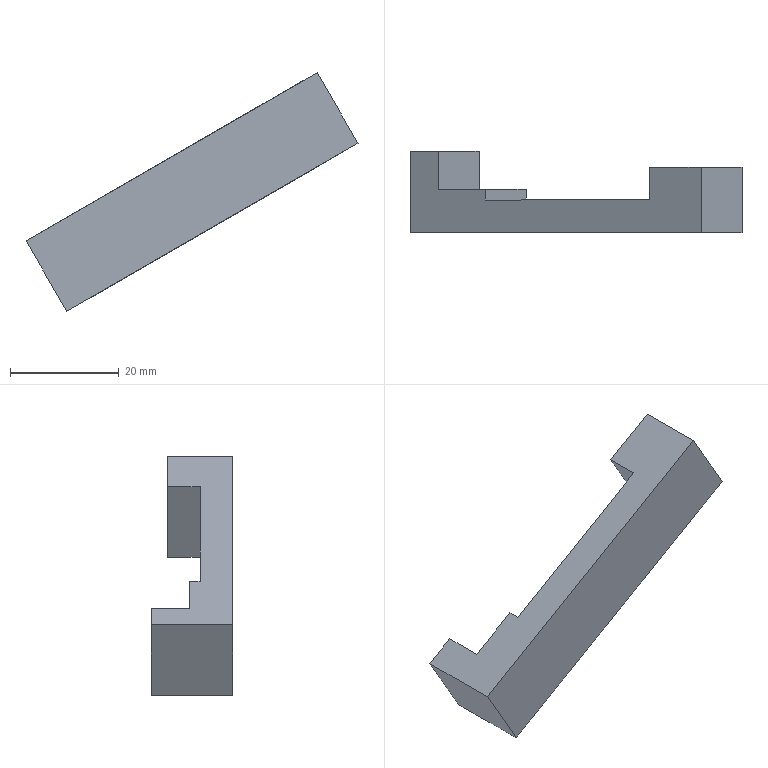Part | NX | features solid 2 | 1 solid | 12 faces | box 61.034 x 15 x 43.898 mm | volume 7663 mm3 | plane 12
STEP:
#1=CARTESIAN_POINT('',(16.962,672.,239.949));
#2=VERTEX_POINT('',#1);
#3=CARTESIAN_POINT('',(9.462,672.,252.94));
#4=VERTEX_POINT('',#3);
#5=CARTESIAN_POINT('',(16.962,672.,239.949));
#6=DIRECTION('',(0.5,0.,-0.866));
#7=VECTOR('',#6,1000.);
#8=LINE('',#5,#7);
#9=EDGE_CURVE('',#2,#4,#8,.F.);
#10=ORIENTED_EDGE('',*,*,#9,.F.);
#11=CARTESIAN_POINT('',(-13.189,672.,222.542));
#12=VERTEX_POINT('',#11);
#13=CARTESIAN_POINT('',(26.488,672.,245.449));
#14=DIRECTION('',(-0.866,0.,-0.5));
#15=VECTOR('',#14,1000.);
#16=LINE('',#13,#15);
#17=EDGE_CURVE('',#2,#12,#16,.T.);
#18=ORIENTED_EDGE('',*,*,#17,.T.);
#19=CARTESIAN_POINT('',(-20.689,672.,235.532));
#20=VERTEX_POINT('',#19);
#21=CARTESIAN_POINT('',(-13.189,672.,222.542));
#22=DIRECTION('',(-0.5,0.,0.866));
#23=VECTOR('',#22,1000.);
#24=LINE('',#21,#23);
#25=EDGE_CURVE('',#12,#20,#24,.T.);
#26=ORIENTED_EDGE('',*,*,#25,.T.);
#27=CARTESIAN_POINT('',(18.988,672.,258.44));
#28=DIRECTION('',(-0.866,0.,-0.5));
#29=VECTOR('',#28,1000.);
#30=LINE('',#27,#29);
#31=EDGE_CURVE('',#4,#20,#30,.T.);
#32=ORIENTED_EDGE('',*,*,#31,.F.);
#33=EDGE_LOOP('',(#10,#18,#26,#32));
#34=FACE_BOUND('',#33,.T.);
#35=CARTESIAN_POINT('',(11.488,672.,271.43));
#36=DIRECTION('',(0.,-1.,0.));
#37=DIRECTION('',(-0.866,0.,-0.5));
#38=AXIS2_PLACEMENT_3D('',#35,#36,#37);
#39=PLANE('',#38);
#40=ADVANCED_FACE('',(#34),#39,.F.);
#41=CARTESIAN_POINT('',(26.488,666.,245.449));
#42=VERTEX_POINT('',#41);
#43=CARTESIAN_POINT('',(18.988,666.,258.44));
#44=VERTEX_POINT('',#43);
#45=CARTESIAN_POINT('',(11.488,666.,271.43));
#46=DIRECTION('',(0.5,0.,-0.866));
#47=VECTOR('',#46,1000.);
#48=LINE('',#45,#47);
#49=EDGE_CURVE('',#42,#44,#48,.F.);
#50=ORIENTED_EDGE('',*,*,#49,.T.);
#51=CARTESIAN_POINT('',(-34.545,666.,227.532));
#52=VERTEX_POINT('',#51);
#53=CARTESIAN_POINT('',(18.988,666.,258.44));
#54=DIRECTION('',(-0.866,0.,-0.5));
#55=VECTOR('',#54,1000.);
#56=LINE('',#53,#55);
#57=EDGE_CURVE('',#44,#52,#56,.T.);
#58=ORIENTED_EDGE('',*,*,#57,.T.);
#59=CARTESIAN_POINT('',(-27.045,666.,214.542));
#60=VERTEX_POINT('',#59);
#61=CARTESIAN_POINT('',(-42.045,666.,240.522));
#62=DIRECTION('',(-0.5,0.,0.866));
#63=VECTOR('',#62,1000.);
#64=LINE('',#61,#63);
#65=EDGE_CURVE('',#60,#52,#64,.T.);
#66=ORIENTED_EDGE('',*,*,#65,.F.);
#67=CARTESIAN_POINT('',(26.488,666.,245.449));
#68=DIRECTION('',(-0.866,0.,-0.5));
#69=VECTOR('',#68,1000.);
#70=LINE('',#67,#69);
#71=EDGE_CURVE('',#42,#60,#70,.T.);
#72=ORIENTED_EDGE('',*,*,#71,.F.);
#73=EDGE_LOOP('',(#50,#58,#66,#72));
#74=FACE_BOUND('',#73,.T.);
#75=CARTESIAN_POINT('',(11.488,666.,271.43));
#76=DIRECTION('',(0.,-1.,0.));
#77=DIRECTION('',(-0.866,0.,-0.5));
#78=AXIS2_PLACEMENT_3D('',#75,#76,#77);
#79=PLANE('',#78);
#80=ADVANCED_FACE('',(#74),#79,.T.);
#81=ORIENTED_EDGE('',*,*,#65,.T.);
#82=CARTESIAN_POINT('',(-34.545,681.,227.532));
#83=VERTEX_POINT('',#82);
#84=CARTESIAN_POINT('',(-34.545,666.,227.532));
#85=DIRECTION('',(0.,-1.,0.));
#86=VECTOR('',#85,1000.);
#87=LINE('',#84,#86);
#88=EDGE_CURVE('',#52,#83,#87,.F.);
#89=ORIENTED_EDGE('',*,*,#88,.T.);
#90=CARTESIAN_POINT('',(-27.045,681.,214.542));
#91=VERTEX_POINT('',#90);
#92=CARTESIAN_POINT('',(-27.045,681.,214.542));
#93=DIRECTION('',(-0.5,0.,0.866));
#94=VECTOR('',#93,1000.);
#95=LINE('',#92,#94);
#96=EDGE_CURVE('',#91,#83,#95,.T.);
#97=ORIENTED_EDGE('',*,*,#96,.F.);
#98=CARTESIAN_POINT('',(-27.045,666.,214.542));
#99=DIRECTION('',(0.,-1.,0.));
#100=VECTOR('',#99,1000.);
#101=LINE('',#98,#100);
#102=EDGE_CURVE('',#60,#91,#101,.F.);
#103=ORIENTED_EDGE('',*,*,#102,.F.);
#104=EDGE_LOOP('',(#81,#89,#97,#103));
#105=FACE_BOUND('',#104,.T.);
#106=CARTESIAN_POINT('',(-42.045,666.,240.522));
#107=DIRECTION('',(-0.866,0.,-0.5));
#108=DIRECTION('',(0.,1.,0.));
#109=AXIS2_PLACEMENT_3D('',#106,#107,#108);
#110=PLANE('',#109);
#111=ADVANCED_FACE('',(#105),#110,.T.);
#112=CARTESIAN_POINT('',(26.488,678.,245.449));
#113=VERTEX_POINT('',#112);
#114=CARTESIAN_POINT('',(26.488,666.,245.449));
#115=DIRECTION('',(0.,1.,0.));
#116=VECTOR('',#115,1000.);
#117=LINE('',#114,#116);
#118=EDGE_CURVE('',#42,#113,#117,.T.);
#119=ORIENTED_EDGE('',*,*,#118,.T.);
#120=CARTESIAN_POINT('',(18.988,678.,258.44));
#121=VERTEX_POINT('',#120);
#122=CARTESIAN_POINT('',(26.488,678.,245.449));
#123=DIRECTION('',(-0.5,0.,0.866));
#124=VECTOR('',#123,1000.);
#125=LINE('',#122,#124);
#126=EDGE_CURVE('',#113,#121,#125,.T.);
#127=ORIENTED_EDGE('',*,*,#126,.T.);
#128=CARTESIAN_POINT('',(18.988,666.,258.44));
#129=DIRECTION('',(0.,1.,0.));
#130=VECTOR('',#129,1000.);
#131=LINE('',#128,#130);
#132=EDGE_CURVE('',#44,#121,#131,.T.);
#133=ORIENTED_EDGE('',*,*,#132,.F.);
#134=ORIENTED_EDGE('',*,*,#49,.F.);
#135=EDGE_LOOP('',(#119,#127,#133,#134));
#136=FACE_BOUND('',#135,.T.);
#137=CARTESIAN_POINT('',(11.488,666.,271.43));
#138=DIRECTION('',(-0.866,0.,-0.5));
#139=DIRECTION('',(0.,1.,0.));
#140=AXIS2_PLACEMENT_3D('',#137,#138,#139);
#141=PLANE('',#140);
#142=ADVANCED_FACE('',(#136),#141,.F.);
#143=CARTESIAN_POINT('',(-29.349,681.,230.532));
#144=VERTEX_POINT('',#143);
#145=CARTESIAN_POINT('',(-29.349,681.,230.532));
#146=DIRECTION('',(-0.866,0.,-0.5));
#147=VECTOR('',#146,1000.);
#148=LINE('',#145,#147);
#149=EDGE_CURVE('',#144,#83,#148,.T.);
#150=ORIENTED_EDGE('',*,*,#149,.T.);
#151=ORIENTED_EDGE('',*,*,#88,.F.);
#152=ORIENTED_EDGE('',*,*,#57,.F.);
#153=ORIENTED_EDGE('',*,*,#132,.T.);
#154=CARTESIAN_POINT('',(9.462,678.,252.94));
#155=VERTEX_POINT('',#154);
#156=CARTESIAN_POINT('',(18.988,678.,258.44));
#157=DIRECTION('',(0.866,0.,0.5));
#158=VECTOR('',#157,1000.);
#159=LINE('',#156,#158);
#160=EDGE_CURVE('',#121,#155,#159,.F.);
#161=ORIENTED_EDGE('',*,*,#160,.T.);
#162=CARTESIAN_POINT('',(9.462,678.,252.94));
#163=DIRECTION('',(0.,1.,0.));
#164=VECTOR('',#163,1000.);
#165=LINE('',#162,#164);
#166=EDGE_CURVE('',#155,#4,#165,.F.);
#167=ORIENTED_EDGE('',*,*,#166,.T.);
#168=ORIENTED_EDGE('',*,*,#31,.T.);
#169=CARTESIAN_POINT('',(-20.689,674.,235.532));
#170=VERTEX_POINT('',#169);
#171=CARTESIAN_POINT('',(-20.689,672.,235.532));
#172=DIRECTION('',(0.,1.,0.));
#173=VECTOR('',#172,1000.);
#174=LINE('',#171,#173);
#175=EDGE_CURVE('',#20,#170,#174,.T.);
#176=ORIENTED_EDGE('',*,*,#175,.T.);
#177=CARTESIAN_POINT('',(-29.349,674.,230.532));
#178=VERTEX_POINT('',#177);
#179=CARTESIAN_POINT('',(-20.689,674.,235.532));
#180=DIRECTION('',(-0.866,0.,-0.5));
#181=VECTOR('',#180,1000.);
#182=LINE('',#179,#181);
#183=EDGE_CURVE('',#170,#178,#182,.T.);
#184=ORIENTED_EDGE('',*,*,#183,.T.);
#185=CARTESIAN_POINT('',(-29.349,672.,230.532));
#186=DIRECTION('',(0.,1.,0.));
#187=VECTOR('',#186,1000.);
#188=LINE('',#185,#187);
#189=EDGE_CURVE('',#178,#144,#188,.T.);
#190=ORIENTED_EDGE('',*,*,#189,.T.);
#191=EDGE_LOOP('',(#150,#151,#152,#153,#161,#167,#168,#176,#184,#190));
#192=FACE_BOUND('',#191,.T.);
#193=CARTESIAN_POINT('',(18.988,666.,258.44));
#194=DIRECTION('',(0.5,0.,-0.866));
#195=DIRECTION('',(-0.866,0.,-0.5));
#196=AXIS2_PLACEMENT_3D('',#193,#194,#195);
#197=PLANE('',#196);
#198=ADVANCED_FACE('',(#192),#197,.F.);
#199=ORIENTED_EDGE('',*,*,#102,.T.);
#200=CARTESIAN_POINT('',(-21.849,681.,217.542));
#201=VERTEX_POINT('',#200);
#202=CARTESIAN_POINT('',(-21.849,681.,217.542));
#203=DIRECTION('',(-0.866,0.,-0.5));
#204=VECTOR('',#203,1000.);
#205=LINE('',#202,#204);
#206=EDGE_CURVE('',#201,#91,#205,.T.);
#207=ORIENTED_EDGE('',*,*,#206,.F.);
#208=CARTESIAN_POINT('',(-21.849,674.,217.542));
#209=VERTEX_POINT('',#208);
#210=CARTESIAN_POINT('',(-21.849,672.,217.542));
#211=DIRECTION('',(0.,1.,0.));
#212=VECTOR('',#211,1000.);
#213=LINE('',#210,#212);
#214=EDGE_CURVE('',#209,#201,#213,.T.);
#215=ORIENTED_EDGE('',*,*,#214,.F.);
#216=CARTESIAN_POINT('',(-13.189,674.,222.542));
#217=VERTEX_POINT('',#216);
#218=CARTESIAN_POINT('',(-13.189,674.,222.542));
#219=DIRECTION('',(-0.866,0.,-0.5));
#220=VECTOR('',#219,1000.);
#221=LINE('',#218,#220);
#222=EDGE_CURVE('',#217,#209,#221,.T.);
#223=ORIENTED_EDGE('',*,*,#222,.F.);
#224=CARTESIAN_POINT('',(-13.189,672.,222.542));
#225=DIRECTION('',(0.,1.,0.));
#226=VECTOR('',#225,1000.);
#227=LINE('',#224,#226);
#228=EDGE_CURVE('',#12,#217,#227,.T.);
#229=ORIENTED_EDGE('',*,*,#228,.F.);
#230=ORIENTED_EDGE('',*,*,#17,.F.);
#231=CARTESIAN_POINT('',(16.962,678.,239.949));
#232=VERTEX_POINT('',#231);
#233=CARTESIAN_POINT('',(16.962,678.,239.949));
#234=DIRECTION('',(0.,1.,0.));
#235=VECTOR('',#234,1000.);
#236=LINE('',#233,#235);
#237=EDGE_CURVE('',#232,#2,#236,.F.);
#238=ORIENTED_EDGE('',*,*,#237,.F.);
#239=CARTESIAN_POINT('',(26.488,678.,245.449));
#240=DIRECTION('',(0.866,0.,0.5));
#241=VECTOR('',#240,1000.);
#242=LINE('',#239,#241);
#243=EDGE_CURVE('',#113,#232,#242,.F.);
#244=ORIENTED_EDGE('',*,*,#243,.F.);
#245=ORIENTED_EDGE('',*,*,#118,.F.);
#246=ORIENTED_EDGE('',*,*,#71,.T.);
#247=EDGE_LOOP('',(#199,#207,#215,#223,#229,#230,#238,#244,#245,#246));
#248=FACE_BOUND('',#247,.T.);
#249=CARTESIAN_POINT('',(26.488,666.,245.449));
#250=DIRECTION('',(0.5,0.,-0.866));
#251=DIRECTION('',(-0.866,0.,-0.5));
#252=AXIS2_PLACEMENT_3D('',#249,#250,#251);
#253=PLANE('',#252);
#254=ADVANCED_FACE('',(#248),#253,.T.);
#255=ORIENTED_EDGE('',*,*,#175,.F.);
#256=ORIENTED_EDGE('',*,*,#25,.F.);
#257=ORIENTED_EDGE('',*,*,#228,.T.);
#258=CARTESIAN_POINT('',(-13.189,674.,222.542));
#259=DIRECTION('',(-0.5,0.,0.866));
#260=VECTOR('',#259,1000.);
#261=LINE('',#258,#260);
#262=EDGE_CURVE('',#217,#170,#261,.T.);
#263=ORIENTED_EDGE('',*,*,#262,.T.);
#264=EDGE_LOOP('',(#255,#256,#257,#263));
#265=FACE_BOUND('',#264,.T.);
#266=CARTESIAN_POINT('',(-13.189,672.,222.542));
#267=DIRECTION('',(0.866,0.,0.5));
#268=DIRECTION('',(-0.5,0.,0.866));
#269=AXIS2_PLACEMENT_3D('',#266,#267,#268);
#270=PLANE('',#269);
#271=ADVANCED_FACE('',(#265),#270,.T.);
#272=CARTESIAN_POINT('',(-21.849,674.,217.542));
#273=DIRECTION('',(-0.5,0.,0.866));
#274=VECTOR('',#273,1000.);
#275=LINE('',#272,#274);
#276=EDGE_CURVE('',#209,#178,#275,.T.);
#277=ORIENTED_EDGE('',*,*,#276,.T.);
#278=ORIENTED_EDGE('',*,*,#183,.F.);
#279=ORIENTED_EDGE('',*,*,#262,.F.);
#280=ORIENTED_EDGE('',*,*,#222,.T.);
#281=EDGE_LOOP('',(#277,#278,#279,#280));
#282=FACE_BOUND('',#281,.T.);
#283=CARTESIAN_POINT('',(-13.189,674.,222.542));
#284=DIRECTION('',(0.,-1.,0.));
#285=DIRECTION('',(0.,0.,-1.));
#286=AXIS2_PLACEMENT_3D('',#283,#284,#285);
#287=PLANE('',#286);
#288=ADVANCED_FACE('',(#282),#287,.F.);
#289=ORIENTED_EDGE('',*,*,#276,.F.);
#290=ORIENTED_EDGE('',*,*,#214,.T.);
#291=CARTESIAN_POINT('',(-21.849,681.,217.542));
#292=DIRECTION('',(-0.5,0.,0.866));
#293=VECTOR('',#292,1000.);
#294=LINE('',#291,#293);
#295=EDGE_CURVE('',#201,#144,#294,.T.);
#296=ORIENTED_EDGE('',*,*,#295,.T.);
#297=ORIENTED_EDGE('',*,*,#189,.F.);
#298=EDGE_LOOP('',(#289,#290,#296,#297));
#299=FACE_BOUND('',#298,.T.);
#300=CARTESIAN_POINT('',(-21.849,672.,217.542));
#301=DIRECTION('',(0.866,0.,0.5));
#302=DIRECTION('',(-0.5,0.,0.866));
#303=AXIS2_PLACEMENT_3D('',#300,#301,#302);
#304=PLANE('',#303);
#305=ADVANCED_FACE('',(#299),#304,.T.);
#306=ORIENTED_EDGE('',*,*,#96,.T.);
#307=ORIENTED_EDGE('',*,*,#149,.F.);
#308=ORIENTED_EDGE('',*,*,#295,.F.);
#309=ORIENTED_EDGE('',*,*,#206,.T.);
#310=EDGE_LOOP('',(#306,#307,#308,#309));
#311=FACE_BOUND('',#310,.T.);
#312=CARTESIAN_POINT('',(-21.849,681.,217.542));
#313=DIRECTION('',(0.,-1.,0.));
#314=DIRECTION('',(0.,0.,-1.));
#315=AXIS2_PLACEMENT_3D('',#312,#313,#314);
#316=PLANE('',#315);
#317=ADVANCED_FACE('',(#311),#316,.F.);
#318=ORIENTED_EDGE('',*,*,#243,.T.);
#319=CARTESIAN_POINT('',(16.962,678.,239.949));
#320=DIRECTION('',(0.5,0.,-0.866));
#321=VECTOR('',#320,1000.);
#322=LINE('',#319,#321);
#323=EDGE_CURVE('',#232,#155,#322,.F.);
#324=ORIENTED_EDGE('',*,*,#323,.T.);
#325=ORIENTED_EDGE('',*,*,#160,.F.);
#326=ORIENTED_EDGE('',*,*,#126,.F.);
#327=EDGE_LOOP('',(#318,#324,#325,#326));
#328=FACE_BOUND('',#327,.T.);
#329=CARTESIAN_POINT('',(26.488,678.,245.449));
#330=DIRECTION('',(0.,1.,0.));
#331=DIRECTION('',(-0.5,0.,0.866));
#332=AXIS2_PLACEMENT_3D('',#329,#330,#331);
#333=PLANE('',#332);
#334=ADVANCED_FACE('',(#328),#333,.T.);
#335=ORIENTED_EDGE('',*,*,#9,.T.);
#336=ORIENTED_EDGE('',*,*,#166,.F.);
#337=ORIENTED_EDGE('',*,*,#323,.F.);
#338=ORIENTED_EDGE('',*,*,#237,.T.);
#339=EDGE_LOOP('',(#335,#336,#337,#338));
#340=FACE_BOUND('',#339,.T.);
#341=CARTESIAN_POINT('',(16.962,678.,239.949));
#342=DIRECTION('',(0.866,0.,0.5));
#343=DIRECTION('',(0.5,0.,-0.866));
#344=AXIS2_PLACEMENT_3D('',#341,#342,#343);
#345=PLANE('',#344);
#346=ADVANCED_FACE('',(#340),#345,.F.);
#347=CLOSED_SHELL('',(#40,#80,#111,#142,#198,#254,#271,#288,#305,#317,#334,#346));
#348=MANIFOLD_SOLID_BREP('',#347);
#349=(LENGTH_UNIT()NAMED_UNIT(*)SI_UNIT(.MILLI.,.METRE.));
#350=UNCERTAINTY_MEASURE_WITH_UNIT(LENGTH_MEASURE(0.00001),#349,'','');
#351=(NAMED_UNIT(*)PLANE_ANGLE_UNIT()SI_UNIT($,.RADIAN.));
#352=(NAMED_UNIT(*)SI_UNIT($,.STERADIAN.)SOLID_ANGLE_UNIT());
#353=(GEOMETRIC_REPRESENTATION_CONTEXT(3)GLOBAL_UNCERTAINTY_ASSIGNED_CONTEXT((#350))GLOBAL_UNIT_ASSIGNED_CONTEXT((#349,#351,#352))REPRESENTATION_CONTEXT('',''));
#354=ADVANCED_BREP_SHAPE_REPRESENTATION('',(#348),#353);